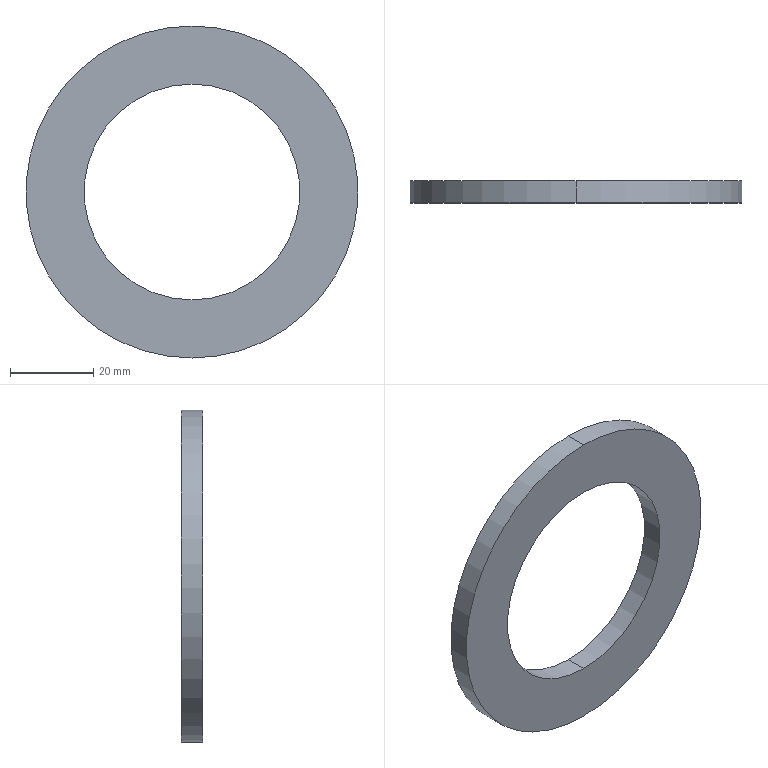Part | SolidWorks | features Extrusion 1 | 1 solid | 6 faces | box 80 x 5.3 x 80 mm | volume 15385 mm3 | cylinder 4 | plane 2 | commonest cylinder face diameters 52 x2 80 x2
STEP:
#1=CARTESIAN_POINT('',(0.,5.3,-26.));
#2=VERTEX_POINT('',#1);
#3=CARTESIAN_POINT('',(0.,5.3,26.));
#4=VERTEX_POINT('',#3);
#5=CARTESIAN_POINT('',(0.,5.3,0.));
#6=DIRECTION('',(0.,1.,0.));
#7=DIRECTION('',(0.,0.,1.));
#8=AXIS2_PLACEMENT_3D('',#5,#6,#7);
#9=CIRCLE('',#8,26.);
#10=EDGE_CURVE('',#2,#4,#9,.T.);
#11=ORIENTED_EDGE('',*,*,#10,.T.);
#12=CARTESIAN_POINT('',(0.,0.,26.));
#13=VERTEX_POINT('',#12);
#14=CARTESIAN_POINT('',(0.,5.3,26.));
#15=DIRECTION('',(0.,-1.,0.));
#16=VECTOR('',#15,1000.);
#17=LINE('',#14,#16);
#18=EDGE_CURVE('',#4,#13,#17,.T.);
#19=ORIENTED_EDGE('',*,*,#18,.T.);
#20=CARTESIAN_POINT('',(0.,0.,-26.));
#21=VERTEX_POINT('',#20);
#22=CARTESIAN_POINT('',(0.,0.,0.));
#23=DIRECTION('',(0.,1.,0.));
#24=DIRECTION('',(0.,0.,1.));
#25=AXIS2_PLACEMENT_3D('',#22,#23,#24);
#26=CIRCLE('',#25,26.);
#27=EDGE_CURVE('',#21,#13,#26,.T.);
#28=ORIENTED_EDGE('',*,*,#27,.F.);
#29=CARTESIAN_POINT('',(0.,5.3,-26.));
#30=DIRECTION('',(0.,-1.,0.));
#31=VECTOR('',#30,1000.);
#32=LINE('',#29,#31);
#33=EDGE_CURVE('',#2,#21,#32,.T.);
#34=ORIENTED_EDGE('',*,*,#33,.F.);
#35=EDGE_LOOP('',(#11,#19,#28,#34));
#36=FACE_OUTER_BOUND('',#35,.T.);
#37=CARTESIAN_POINT('',(0.,5.3,0.));
#38=DIRECTION('',(0.,-1.,0.));
#39=DIRECTION('',(0.,0.,-1.));
#40=AXIS2_PLACEMENT_3D('',#37,#38,#39);
#41=CYLINDRICAL_SURFACE('',#40,26.);
#42=ADVANCED_FACE('',(#36),#41,.F.);
#43=CARTESIAN_POINT('',(0.,5.3,40.));
#44=VERTEX_POINT('',#43);
#45=CARTESIAN_POINT('',(0.,5.3,-40.));
#46=VERTEX_POINT('',#45);
#47=CARTESIAN_POINT('',(0.,5.3,0.));
#48=DIRECTION('',(0.,1.,0.));
#49=DIRECTION('',(0.,0.,1.));
#50=AXIS2_PLACEMENT_3D('',#47,#48,#49);
#51=CIRCLE('',#50,40.);
#52=EDGE_CURVE('',#44,#46,#51,.T.);
#53=ORIENTED_EDGE('',*,*,#52,.F.);
#54=CARTESIAN_POINT('',(0.,0.,40.));
#55=VERTEX_POINT('',#54);
#56=CARTESIAN_POINT('',(0.,5.3,40.));
#57=DIRECTION('',(0.,-1.,0.));
#58=VECTOR('',#57,1000.);
#59=LINE('',#56,#58);
#60=EDGE_CURVE('',#44,#55,#59,.T.);
#61=ORIENTED_EDGE('',*,*,#60,.T.);
#62=CARTESIAN_POINT('',(0.,0.,-40.));
#63=VERTEX_POINT('',#62);
#64=CARTESIAN_POINT('',(0.,0.,0.));
#65=DIRECTION('',(0.,1.,0.));
#66=DIRECTION('',(0.,0.,1.));
#67=AXIS2_PLACEMENT_3D('',#64,#65,#66);
#68=CIRCLE('',#67,40.);
#69=EDGE_CURVE('',#55,#63,#68,.T.);
#70=ORIENTED_EDGE('',*,*,#69,.T.);
#71=CARTESIAN_POINT('',(0.,5.3,-40.));
#72=DIRECTION('',(0.,-1.,0.));
#73=VECTOR('',#72,1000.);
#74=LINE('',#71,#73);
#75=EDGE_CURVE('',#46,#63,#74,.T.);
#76=ORIENTED_EDGE('',*,*,#75,.F.);
#77=EDGE_LOOP('',(#53,#61,#70,#76));
#78=FACE_OUTER_BOUND('',#77,.T.);
#79=CARTESIAN_POINT('',(0.,5.3,0.));
#80=DIRECTION('',(0.,-1.,0.));
#81=DIRECTION('',(0.,0.,-1.));
#82=AXIS2_PLACEMENT_3D('',#79,#80,#81);
#83=CYLINDRICAL_SURFACE('',#82,40.);
#84=ADVANCED_FACE('',(#78),#83,.T.);
#85=CARTESIAN_POINT('',(0.,5.3,0.));
#86=DIRECTION('',(0.,1.,0.));
#87=DIRECTION('',(0.,0.,1.));
#88=AXIS2_PLACEMENT_3D('',#85,#86,#87);
#89=CIRCLE('',#88,40.);
#90=EDGE_CURVE('',#46,#44,#89,.T.);
#91=ORIENTED_EDGE('',*,*,#90,.T.);
#92=ORIENTED_EDGE('',*,*,#52,.T.);
#93=EDGE_LOOP('',(#91,#92));
#94=FACE_OUTER_BOUND('',#93,.T.);
#95=ORIENTED_EDGE('',*,*,#10,.F.);
#96=CARTESIAN_POINT('',(0.,5.3,0.));
#97=DIRECTION('',(0.,1.,0.));
#98=DIRECTION('',(0.,0.,1.));
#99=AXIS2_PLACEMENT_3D('',#96,#97,#98);
#100=CIRCLE('',#99,26.);
#101=EDGE_CURVE('',#4,#2,#100,.T.);
#102=ORIENTED_EDGE('',*,*,#101,.F.);
#103=EDGE_LOOP('',(#95,#102));
#104=FACE_BOUND('',#103,.T.);
#105=CARTESIAN_POINT('',(0.,5.3,0.));
#106=DIRECTION('',(0.,1.,0.));
#107=DIRECTION('',(0.,0.,1.));
#108=AXIS2_PLACEMENT_3D('',#105,#106,#107);
#109=PLANE('',#108);
#110=ADVANCED_FACE('',(#94,#104),#109,.T.);
#111=CARTESIAN_POINT('',(0.,0.,0.));
#112=DIRECTION('',(0.,1.,0.));
#113=DIRECTION('',(0.,0.,1.));
#114=AXIS2_PLACEMENT_3D('',#111,#112,#113);
#115=CIRCLE('',#114,40.);
#116=EDGE_CURVE('',#63,#55,#115,.T.);
#117=ORIENTED_EDGE('',*,*,#116,.F.);
#118=ORIENTED_EDGE('',*,*,#69,.F.);
#119=EDGE_LOOP('',(#117,#118));
#120=FACE_OUTER_BOUND('',#119,.T.);
#121=ORIENTED_EDGE('',*,*,#27,.T.);
#122=CARTESIAN_POINT('',(0.,0.,0.));
#123=DIRECTION('',(0.,1.,0.));
#124=DIRECTION('',(0.,0.,1.));
#125=AXIS2_PLACEMENT_3D('',#122,#123,#124);
#126=CIRCLE('',#125,26.);
#127=EDGE_CURVE('',#13,#21,#126,.T.);
#128=ORIENTED_EDGE('',*,*,#127,.T.);
#129=EDGE_LOOP('',(#121,#128));
#130=FACE_BOUND('',#129,.T.);
#131=CARTESIAN_POINT('',(0.,0.,0.));
#132=DIRECTION('',(0.,1.,0.));
#133=DIRECTION('',(0.,0.,1.));
#134=AXIS2_PLACEMENT_3D('',#131,#132,#133);
#135=PLANE('',#134);
#136=ADVANCED_FACE('',(#120,#130),#135,.F.);
#137=ORIENTED_EDGE('',*,*,#60,.F.);
#138=ORIENTED_EDGE('',*,*,#90,.F.);
#139=ORIENTED_EDGE('',*,*,#75,.T.);
#140=ORIENTED_EDGE('',*,*,#116,.T.);
#141=EDGE_LOOP('',(#137,#138,#139,#140));
#142=FACE_OUTER_BOUND('',#141,.T.);
#143=CARTESIAN_POINT('',(0.,5.3,0.));
#144=DIRECTION('',(0.,-1.,0.));
#145=DIRECTION('',(0.,0.,-1.));
#146=AXIS2_PLACEMENT_3D('',#143,#144,#145);
#147=CYLINDRICAL_SURFACE('',#146,40.);
#148=ADVANCED_FACE('',(#142),#147,.T.);
#149=ORIENTED_EDGE('',*,*,#18,.F.);
#150=ORIENTED_EDGE('',*,*,#101,.T.);
#151=ORIENTED_EDGE('',*,*,#33,.T.);
#152=ORIENTED_EDGE('',*,*,#127,.F.);
#153=EDGE_LOOP('',(#149,#150,#151,#152));
#154=FACE_OUTER_BOUND('',#153,.T.);
#155=CARTESIAN_POINT('',(0.,5.3,0.));
#156=DIRECTION('',(0.,-1.,0.));
#157=DIRECTION('',(0.,0.,-1.));
#158=AXIS2_PLACEMENT_3D('',#155,#156,#157);
#159=CYLINDRICAL_SURFACE('',#158,26.);
#160=ADVANCED_FACE('',(#154),#159,.F.);
#161=CLOSED_SHELL('',(#42,#84,#110,#136,#148,#160));
#162=MANIFOLD_SOLID_BREP('',#161);
#163=CARTESIAN_POINT('',(0.,0.,0.));
#164=DIRECTION('',(0.,0.,1.));
#165=DIRECTION('',(1.,0.,0.));
#166=AXIS2_PLACEMENT_3D('',#163,#164,#165);
#167=(LENGTH_UNIT()NAMED_UNIT(*)SI_UNIT(.MILLI.,.METRE.));
#168=UNCERTAINTY_MEASURE_WITH_UNIT(LENGTH_MEASURE(0.00001),#167,'','');
#169=(NAMED_UNIT(*)PLANE_ANGLE_UNIT()SI_UNIT($,.RADIAN.));
#170=(NAMED_UNIT(*)SI_UNIT($,.STERADIAN.)SOLID_ANGLE_UNIT());
#171=(GEOMETRIC_REPRESENTATION_CONTEXT(3)GLOBAL_UNCERTAINTY_ASSIGNED_CONTEXT((#168))GLOBAL_UNIT_ASSIGNED_CONTEXT((#167,#169,#170))REPRESENTATION_CONTEXT('',''));
#172=ADVANCED_BREP_SHAPE_REPRESENTATION('',(#162,#166),#171);